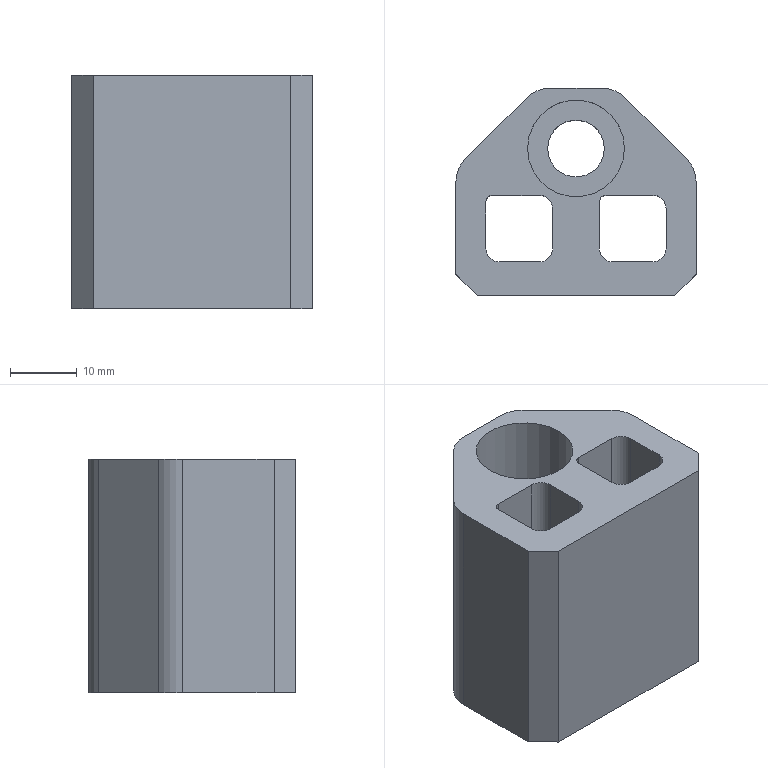Part | NX | features DIE-87 2 | 1 solid | 41 faces | box 36 x 31 x 35 mm | volume 23425 mm3 | plane 23 | cylinder 18 | commonest cylinder face diameters 4 x6 6 x4 10 x4 2 x2 8.5 x1 14.5 x1
STEP:
#1=CARTESIAN_POINT('',(4075.486,-827.123,823.716));
#2=VERTEX_POINT('',#1);
#3=CARTESIAN_POINT('',(4079.736,-827.123,823.716));
#4=DIRECTION('',(0.,0.,1.));
#5=DIRECTION('',(-1.,0.,0.));
#6=AXIS2_PLACEMENT_3D('',#3,#4,#5);
#7=CIRCLE('',#6,4.25);
#8=EDGE_CURVE('',#2,#2,#7,.T.);
#9=ORIENTED_EDGE('',*,*,#8,.T.);
#10=EDGE_LOOP('',(#9));
#11=FACE_BOUND('',#10,.T.);
#12=CARTESIAN_POINT('',(4072.272,-819.587,823.716));
#13=VERTEX_POINT('',#12);
#14=CARTESIAN_POINT('',(4063.201,-828.658,823.716));
#15=VERTEX_POINT('',#14);
#16=CARTESIAN_POINT('',(4078.661,-813.198,823.716));
#17=DIRECTION('',(-0.7071,-0.7071,0.));
#18=VECTOR('',#17,1000.);
#19=LINE('',#16,#18);
#20=EDGE_CURVE('',#13,#15,#19,.T.);
#21=ORIENTED_EDGE('',*,*,#20,.F.);
#22=CARTESIAN_POINT('',(4075.807,-818.123,823.716));
#23=VERTEX_POINT('',#22);
#24=CARTESIAN_POINT('',(4075.807,-823.123,823.716));
#25=DIRECTION('',(0.,0.,1.));
#26=DIRECTION('',(-1.,0.,0.));
#27=AXIS2_PLACEMENT_3D('',#24,#25,#26);
#28=CIRCLE('',#27,5.);
#29=EDGE_CURVE('',#23,#13,#28,.T.);
#30=ORIENTED_EDGE('',*,*,#29,.F.);
#31=CARTESIAN_POINT('',(4083.665,-818.123,823.716));
#32=VERTEX_POINT('',#31);
#33=CARTESIAN_POINT('',(4123.586,-818.123,823.716));
#34=DIRECTION('',(1.,0.,0.));
#35=VECTOR('',#34,1000.);
#36=LINE('',#33,#35);
#37=EDGE_CURVE('',#23,#32,#36,.T.);
#38=ORIENTED_EDGE('',*,*,#37,.T.);
#39=CARTESIAN_POINT('',(4087.201,-819.587,823.716));
#40=VERTEX_POINT('',#39);
#41=CARTESIAN_POINT('',(4083.665,-823.123,823.716));
#42=DIRECTION('',(0.,0.,1.));
#43=DIRECTION('',(-1.,0.,0.));
#44=AXIS2_PLACEMENT_3D('',#41,#42,#43);
#45=CIRCLE('',#44,5.);
#46=EDGE_CURVE('',#40,#32,#45,.T.);
#47=ORIENTED_EDGE('',*,*,#46,.F.);
#48=CARTESIAN_POINT('',(4096.272,-828.658,823.716));
#49=VERTEX_POINT('',#48);
#50=CARTESIAN_POINT('',(4124.661,-857.048,823.716));
#51=DIRECTION('',(-0.7071,0.7071,0.));
#52=VECTOR('',#51,1000.);
#53=LINE('',#50,#52);
#54=EDGE_CURVE('',#49,#40,#53,.T.);
#55=ORIENTED_EDGE('',*,*,#54,.F.);
#56=CARTESIAN_POINT('',(4097.736,-832.194,823.716));
#57=VERTEX_POINT('',#56);
#58=CARTESIAN_POINT('',(4092.736,-832.194,823.716));
#59=DIRECTION('',(0.,0.,1.));
#60=DIRECTION('',(-1.,0.,0.));
#61=AXIS2_PLACEMENT_3D('',#58,#59,#60);
#62=CIRCLE('',#61,5.);
#63=EDGE_CURVE('',#57,#49,#62,.T.);
#64=ORIENTED_EDGE('',*,*,#63,.F.);
#65=CARTESIAN_POINT('',(4097.736,-845.923,823.716));
#66=VERTEX_POINT('',#65);
#67=CARTESIAN_POINT('',(4097.736,-858.123,823.716));
#68=DIRECTION('',(0.,-1.,0.));
#69=VECTOR('',#68,1000.);
#70=LINE('',#67,#69);
#71=EDGE_CURVE('',#57,#66,#70,.T.);
#72=ORIENTED_EDGE('',*,*,#71,.T.);
#73=CARTESIAN_POINT('',(4094.536,-849.123,823.716));
#74=VERTEX_POINT('',#73);
#75=CARTESIAN_POINT('',(4104.561,-839.098,823.716));
#76=DIRECTION('',(-0.7071,-0.7071,0.));
#77=VECTOR('',#76,1000.);
#78=LINE('',#75,#77);
#79=EDGE_CURVE('',#74,#66,#78,.F.);
#80=ORIENTED_EDGE('',*,*,#79,.F.);
#81=CARTESIAN_POINT('',(4064.936,-849.123,823.716));
#82=VERTEX_POINT('',#81);
#83=CARTESIAN_POINT('',(4123.586,-849.123,823.716));
#84=DIRECTION('',(1.,0.,0.));
#85=VECTOR('',#84,1000.);
#86=LINE('',#83,#85);
#87=EDGE_CURVE('',#82,#74,#86,.T.);
#88=ORIENTED_EDGE('',*,*,#87,.F.);
#89=CARTESIAN_POINT('',(4061.736,-845.923,823.716));
#90=VERTEX_POINT('',#89);
#91=CARTESIAN_POINT('',(4098.761,-882.948,823.716));
#92=DIRECTION('',(-0.7071,0.7071,0.));
#93=VECTOR('',#92,1000.);
#94=LINE('',#91,#93);
#95=EDGE_CURVE('',#90,#82,#94,.F.);
#96=ORIENTED_EDGE('',*,*,#95,.F.);
#97=CARTESIAN_POINT('',(4061.736,-832.194,823.716));
#98=VERTEX_POINT('',#97);
#99=CARTESIAN_POINT('',(4061.736,-858.123,823.716));
#100=DIRECTION('',(0.,1.,0.));
#101=VECTOR('',#100,1000.);
#102=LINE('',#99,#101);
#103=EDGE_CURVE('',#90,#98,#102,.T.);
#104=ORIENTED_EDGE('',*,*,#103,.T.);
#105=CARTESIAN_POINT('',(4066.736,-832.194,823.716));
#106=DIRECTION('',(0.,0.,1.));
#107=DIRECTION('',(-1.,0.,0.));
#108=AXIS2_PLACEMENT_3D('',#105,#106,#107);
#109=CIRCLE('',#108,5.);
#110=EDGE_CURVE('',#15,#98,#109,.T.);
#111=ORIENTED_EDGE('',*,*,#110,.F.);
#112=EDGE_LOOP('',(#21,#30,#38,#47,#55,#64,#72,#80,#88,#96,#104,#111));
#113=FACE_BOUND('',#112,.T.);
#114=CARTESIAN_POINT('',(4095.236,-841.123,823.716));
#115=VERTEX_POINT('',#114);
#116=CARTESIAN_POINT('',(4095.236,-837.123,823.716));
#117=VERTEX_POINT('',#116);
#118=CARTESIAN_POINT('',(4095.236,-841.123,823.716));
#119=DIRECTION('',(0.,1.,0.));
#120=VECTOR('',#119,1000.);
#121=LINE('',#118,#120);
#122=EDGE_CURVE('',#115,#117,#121,.T.);
#123=ORIENTED_EDGE('',*,*,#122,.T.);
#124=CARTESIAN_POINT('',(4091.685,-834.174,823.716));
#125=VERTEX_POINT('',#124);
#126=CARTESIAN_POINT('',(4092.236,-837.123,823.716));
#127=DIRECTION('',(0.,0.,1.));
#128=DIRECTION('',(1.,0.,0.));
#129=AXIS2_PLACEMENT_3D('',#126,#127,#128);
#130=CIRCLE('',#129,3.);
#131=EDGE_CURVE('',#117,#125,#130,.T.);
#132=ORIENTED_EDGE('',*,*,#131,.T.);
#133=CARTESIAN_POINT('',(4091.236,-834.123,823.716));
#134=VERTEX_POINT('',#133);
#135=CARTESIAN_POINT('',(4091.236,-836.123,823.716));
#136=DIRECTION('',(0.,0.,-1.));
#137=DIRECTION('',(-1.,0.,0.));
#138=AXIS2_PLACEMENT_3D('',#135,#136,#137);
#139=CIRCLE('',#138,2.);
#140=EDGE_CURVE('',#134,#125,#139,.T.);
#141=ORIENTED_EDGE('',*,*,#140,.F.);
#142=CARTESIAN_POINT('',(4084.236,-834.123,823.716));
#143=VERTEX_POINT('',#142);
#144=CARTESIAN_POINT('',(4088.236,-834.123,823.716));
#145=DIRECTION('',(-1.,0.,0.));
#146=VECTOR('',#145,1000.);
#147=LINE('',#144,#146);
#148=EDGE_CURVE('',#134,#143,#147,.T.);
#149=ORIENTED_EDGE('',*,*,#148,.T.);
#150=CARTESIAN_POINT('',(4083.236,-835.123,823.716));
#151=VERTEX_POINT('',#150);
#152=CARTESIAN_POINT('',(4084.236,-835.123,823.716));
#153=DIRECTION('',(0.,0.,-1.));
#154=DIRECTION('',(-1.,0.,0.));
#155=AXIS2_PLACEMENT_3D('',#152,#153,#154);
#156=CIRCLE('',#155,1.);
#157=EDGE_CURVE('',#151,#143,#156,.T.);
#158=ORIENTED_EDGE('',*,*,#157,.F.);
#159=CARTESIAN_POINT('',(4083.236,-842.123,823.716));
#160=VERTEX_POINT('',#159);
#161=CARTESIAN_POINT('',(4083.236,-839.123,823.716));
#162=DIRECTION('',(0.,-1.,0.));
#163=VECTOR('',#162,1000.);
#164=LINE('',#161,#163);
#165=EDGE_CURVE('',#151,#160,#164,.T.);
#166=ORIENTED_EDGE('',*,*,#165,.T.);
#167=CARTESIAN_POINT('',(4085.236,-844.123,823.716));
#168=VERTEX_POINT('',#167);
#169=CARTESIAN_POINT('',(4085.236,-842.123,823.716));
#170=DIRECTION('',(0.,0.,-1.));
#171=DIRECTION('',(-1.,0.,0.));
#172=AXIS2_PLACEMENT_3D('',#169,#170,#171);
#173=CIRCLE('',#172,2.);
#174=EDGE_CURVE('',#168,#160,#173,.T.);
#175=ORIENTED_EDGE('',*,*,#174,.F.);
#176=CARTESIAN_POINT('',(4091.236,-844.123,823.716));
#177=VERTEX_POINT('',#176);
#178=CARTESIAN_POINT('',(4088.236,-844.123,823.716));
#179=DIRECTION('',(1.,0.,0.));
#180=VECTOR('',#179,1000.);
#181=LINE('',#178,#180);
#182=EDGE_CURVE('',#168,#177,#181,.T.);
#183=ORIENTED_EDGE('',*,*,#182,.T.);
#184=CARTESIAN_POINT('',(4091.685,-844.072,823.716));
#185=VERTEX_POINT('',#184);
#186=CARTESIAN_POINT('',(4091.236,-842.123,823.716));
#187=DIRECTION('',(0.,0.,-1.));
#188=DIRECTION('',(-1.,0.,0.));
#189=AXIS2_PLACEMENT_3D('',#186,#187,#188);
#190=CIRCLE('',#189,2.);
#191=EDGE_CURVE('',#185,#177,#190,.T.);
#192=ORIENTED_EDGE('',*,*,#191,.F.);
#193=CARTESIAN_POINT('',(4092.236,-841.123,823.716));
#194=DIRECTION('',(0.,0.,1.));
#195=DIRECTION('',(1.,0.,0.));
#196=AXIS2_PLACEMENT_3D('',#193,#194,#195);
#197=CIRCLE('',#196,3.);
#198=EDGE_CURVE('',#185,#115,#197,.T.);
#199=ORIENTED_EDGE('',*,*,#198,.T.);
#200=EDGE_LOOP('',(#123,#132,#141,#149,#158,#166,#175,#183,#192,#199));
#201=FACE_BOUND('',#200,.T.);
#202=CARTESIAN_POINT('',(4078.236,-841.123,823.716));
#203=VERTEX_POINT('',#202);
#204=CARTESIAN_POINT('',(4078.236,-837.123,823.716));
#205=VERTEX_POINT('',#204);
#206=CARTESIAN_POINT('',(4078.236,-841.123,823.716));
#207=DIRECTION('',(0.,1.,0.));
#208=VECTOR('',#207,1000.);
#209=LINE('',#206,#208);
#210=EDGE_CURVE('',#203,#205,#209,.T.);
#211=ORIENTED_EDGE('',*,*,#210,.T.);
#212=CARTESIAN_POINT('',(4074.685,-834.174,823.716));
#213=VERTEX_POINT('',#212);
#214=CARTESIAN_POINT('',(4075.236,-837.123,823.716));
#215=DIRECTION('',(0.,0.,1.));
#216=DIRECTION('',(1.,0.,0.));
#217=AXIS2_PLACEMENT_3D('',#214,#215,#216);
#218=CIRCLE('',#217,3.);
#219=EDGE_CURVE('',#205,#213,#218,.T.);
#220=ORIENTED_EDGE('',*,*,#219,.T.);
#221=CARTESIAN_POINT('',(4074.236,-834.123,823.716));
#222=VERTEX_POINT('',#221);
#223=CARTESIAN_POINT('',(4074.236,-836.123,823.716));
#224=DIRECTION('',(0.,0.,-1.));
#225=DIRECTION('',(-1.,0.,0.));
#226=AXIS2_PLACEMENT_3D('',#223,#224,#225);
#227=CIRCLE('',#226,2.);
#228=EDGE_CURVE('',#222,#213,#227,.T.);
#229=ORIENTED_EDGE('',*,*,#228,.F.);
#230=CARTESIAN_POINT('',(4067.236,-834.123,823.716));
#231=VERTEX_POINT('',#230);
#232=CARTESIAN_POINT('',(4071.236,-834.123,823.716));
#233=DIRECTION('',(-1.,0.,0.));
#234=VECTOR('',#233,1000.);
#235=LINE('',#232,#234);
#236=EDGE_CURVE('',#222,#231,#235,.T.);
#237=ORIENTED_EDGE('',*,*,#236,.T.);
#238=CARTESIAN_POINT('',(4066.236,-835.123,823.716));
#239=VERTEX_POINT('',#238);
#240=CARTESIAN_POINT('',(4067.236,-835.123,823.716));
#241=DIRECTION('',(0.,0.,-1.));
#242=DIRECTION('',(-1.,0.,0.));
#243=AXIS2_PLACEMENT_3D('',#240,#241,#242);
#244=CIRCLE('',#243,1.);
#245=EDGE_CURVE('',#239,#231,#244,.T.);
#246=ORIENTED_EDGE('',*,*,#245,.F.);
#247=CARTESIAN_POINT('',(4066.236,-842.123,823.716));
#248=VERTEX_POINT('',#247);
#249=CARTESIAN_POINT('',(4066.236,-839.123,823.716));
#250=DIRECTION('',(0.,-1.,0.));
#251=VECTOR('',#250,1000.);
#252=LINE('',#249,#251);
#253=EDGE_CURVE('',#239,#248,#252,.T.);
#254=ORIENTED_EDGE('',*,*,#253,.T.);
#255=CARTESIAN_POINT('',(4068.236,-844.123,823.716));
#256=VERTEX_POINT('',#255);
#257=CARTESIAN_POINT('',(4068.236,-842.123,823.716));
#258=DIRECTION('',(0.,0.,-1.));
#259=DIRECTION('',(-1.,0.,0.));
#260=AXIS2_PLACEMENT_3D('',#257,#258,#259);
#261=CIRCLE('',#260,2.);
#262=EDGE_CURVE('',#256,#248,#261,.T.);
#263=ORIENTED_EDGE('',*,*,#262,.F.);
#264=CARTESIAN_POINT('',(4074.236,-844.123,823.716));
#265=VERTEX_POINT('',#264);
#266=CARTESIAN_POINT('',(4071.236,-844.123,823.716));
#267=DIRECTION('',(1.,0.,0.));
#268=VECTOR('',#267,1000.);
#269=LINE('',#266,#268);
#270=EDGE_CURVE('',#256,#265,#269,.T.);
#271=ORIENTED_EDGE('',*,*,#270,.T.);
#272=CARTESIAN_POINT('',(4074.685,-844.072,823.716));
#273=VERTEX_POINT('',#272);
#274=CARTESIAN_POINT('',(4074.236,-842.123,823.716));
#275=DIRECTION('',(0.,0.,-1.));
#276=DIRECTION('',(-1.,0.,0.));
#277=AXIS2_PLACEMENT_3D('',#274,#275,#276);
#278=CIRCLE('',#277,2.);
#279=EDGE_CURVE('',#273,#265,#278,.T.);
#280=ORIENTED_EDGE('',*,*,#279,.F.);
#281=CARTESIAN_POINT('',(4075.236,-841.123,823.716));
#282=DIRECTION('',(0.,0.,1.));
#283=DIRECTION('',(1.,0.,0.));
#284=AXIS2_PLACEMENT_3D('',#281,#282,#283);
#285=CIRCLE('',#284,3.);
#286=EDGE_CURVE('',#273,#203,#285,.T.);
#287=ORIENTED_EDGE('',*,*,#286,.T.);
#288=EDGE_LOOP('',(#211,#220,#229,#237,#246,#254,#263,#271,#280,#287));
#289=FACE_BOUND('',#288,.T.);
#290=CARTESIAN_POINT('',(4123.586,-858.123,823.716));
#291=DIRECTION('',(0.,0.,-1.));
#292=DIRECTION('',(-1.,0.,0.));
#293=AXIS2_PLACEMENT_3D('',#290,#291,#292);
#294=PLANE('',#293);
#295=ADVANCED_FACE('',(#11,#113,#201,#289),#294,.T.);
#296=CARTESIAN_POINT('',(4074.685,-834.174,828.716));
#297=VERTEX_POINT('',#296);
#298=CARTESIAN_POINT('',(4074.685,-834.174,826.216));
#299=DIRECTION('',(0.,0.,-1.));
#300=VECTOR('',#299,1000.);
#301=LINE('',#298,#300);
#302=EDGE_CURVE('',#297,#213,#301,.T.);
#303=ORIENTED_EDGE('',*,*,#302,.F.);
#304=CARTESIAN_POINT('',(4076.236,-836.123,828.716));
#305=VERTEX_POINT('',#304);
#306=CARTESIAN_POINT('',(4074.236,-836.123,828.716));
#307=DIRECTION('',(0.,0.,1.));
#308=DIRECTION('',(1.,0.,0.));
#309=AXIS2_PLACEMENT_3D('',#306,#307,#308);
#310=CIRCLE('',#309,2.);
#311=EDGE_CURVE('',#297,#305,#310,.F.);
#312=ORIENTED_EDGE('',*,*,#311,.T.);
#313=CARTESIAN_POINT('',(4076.236,-836.123,858.716));
#314=VERTEX_POINT('',#313);
#315=CARTESIAN_POINT('',(4076.236,-836.123,823.716));
#316=DIRECTION('',(0.,0.,1.));
#317=VECTOR('',#316,1000.);
#318=LINE('',#315,#317);
#319=EDGE_CURVE('',#314,#305,#318,.F.);
#320=ORIENTED_EDGE('',*,*,#319,.F.);
#321=CARTESIAN_POINT('',(4074.236,-834.123,858.716));
#322=VERTEX_POINT('',#321);
#323=CARTESIAN_POINT('',(4074.236,-836.123,858.716));
#324=DIRECTION('',(0.,0.,1.));
#325=DIRECTION('',(1.,0.,0.));
#326=AXIS2_PLACEMENT_3D('',#323,#324,#325);
#327=CIRCLE('',#326,2.);
#328=EDGE_CURVE('',#314,#322,#327,.T.);
#329=ORIENTED_EDGE('',*,*,#328,.T.);
#330=CARTESIAN_POINT('',(4074.236,-834.123,823.716));
#331=DIRECTION('',(0.,0.,1.));
#332=VECTOR('',#331,1000.);
#333=LINE('',#330,#332);
#334=EDGE_CURVE('',#222,#322,#333,.T.);
#335=ORIENTED_EDGE('',*,*,#334,.F.);
#336=ORIENTED_EDGE('',*,*,#228,.T.);
#337=EDGE_LOOP('',(#303,#312,#320,#329,#335,#336));
#338=FACE_BOUND('',#337,.T.);
#339=CARTESIAN_POINT('',(4074.236,-836.123,823.716));
#340=DIRECTION('',(0.,0.,1.));
#341=DIRECTION('',(1.,0.,0.));
#342=AXIS2_PLACEMENT_3D('',#339,#340,#341);
#343=CYLINDRICAL_SURFACE('',#342,2.);
#344=ADVANCED_FACE('',(#338),#343,.F.);
#345=CARTESIAN_POINT('',(4074.685,-844.072,828.716));
#346=VERTEX_POINT('',#345);
#347=CARTESIAN_POINT('',(4074.685,-844.072,826.216));
#348=DIRECTION('',(0.,0.,-1.));
#349=VECTOR('',#348,1000.);
#350=LINE('',#347,#349);
#351=EDGE_CURVE('',#273,#346,#350,.F.);
#352=ORIENTED_EDGE('',*,*,#351,.F.);
#353=ORIENTED_EDGE('',*,*,#279,.T.);
#354=CARTESIAN_POINT('',(4074.236,-844.123,858.716));
#355=VERTEX_POINT('',#354);
#356=CARTESIAN_POINT('',(4074.236,-844.123,823.716));
#357=DIRECTION('',(0.,0.,1.));
#358=VECTOR('',#357,1000.);
#359=LINE('',#356,#358);
#360=EDGE_CURVE('',#355,#265,#359,.F.);
#361=ORIENTED_EDGE('',*,*,#360,.F.);
#362=CARTESIAN_POINT('',(4076.236,-842.123,858.716));
#363=VERTEX_POINT('',#362);
#364=CARTESIAN_POINT('',(4074.236,-842.123,858.716));
#365=DIRECTION('',(0.,0.,1.));
#366=DIRECTION('',(1.,0.,0.));
#367=AXIS2_PLACEMENT_3D('',#364,#365,#366);
#368=CIRCLE('',#367,2.);
#369=EDGE_CURVE('',#355,#363,#368,.T.);
#370=ORIENTED_EDGE('',*,*,#369,.T.);
#371=CARTESIAN_POINT('',(4076.236,-842.123,828.716));
#372=VERTEX_POINT('',#371);
#373=CARTESIAN_POINT('',(4076.236,-842.123,823.716));
#374=DIRECTION('',(0.,0.,1.));
#375=VECTOR('',#374,1000.);
#376=LINE('',#373,#375);
#377=EDGE_CURVE('',#372,#363,#376,.T.);
#378=ORIENTED_EDGE('',*,*,#377,.F.);
#379=CARTESIAN_POINT('',(4074.236,-842.123,828.716));
#380=DIRECTION('',(0.,0.,1.));
#381=DIRECTION('',(1.,0.,0.));
#382=AXIS2_PLACEMENT_3D('',#379,#380,#381);
#383=CIRCLE('',#382,2.);
#384=EDGE_CURVE('',#372,#346,#383,.F.);
#385=ORIENTED_EDGE('',*,*,#384,.T.);
#386=EDGE_LOOP('',(#352,#353,#361,#370,#378,#385));
#387=FACE_BOUND('',#386,.T.);
#388=CARTESIAN_POINT('',(4074.236,-842.123,823.716));
#389=DIRECTION('',(0.,0.,1.));
#390=DIRECTION('',(1.,0.,0.));
#391=AXIS2_PLACEMENT_3D('',#388,#389,#390);
#392=CYLINDRICAL_SURFACE('',#391,2.);
#393=ADVANCED_FACE('',(#387),#392,.F.);
#394=CARTESIAN_POINT('',(4091.685,-834.174,828.716));
#395=VERTEX_POINT('',#394);
#396=CARTESIAN_POINT('',(4091.685,-834.174,826.216));
#397=DIRECTION('',(0.,0.,-1.));
#398=VECTOR('',#397,1000.);
#399=LINE('',#396,#398);
#400=EDGE_CURVE('',#395,#125,#399,.T.);
#401=ORIENTED_EDGE('',*,*,#400,.F.);
#402=CARTESIAN_POINT('',(4093.236,-836.123,828.716));
#403=VERTEX_POINT('',#402);
#404=CARTESIAN_POINT('',(4091.236,-836.123,828.716));
#405=DIRECTION('',(0.,0.,1.));
#406=DIRECTION('',(1.,0.,0.));
#407=AXIS2_PLACEMENT_3D('',#404,#405,#406);
#408=CIRCLE('',#407,2.);
#409=EDGE_CURVE('',#395,#403,#408,.F.);
#410=ORIENTED_EDGE('',*,*,#409,.T.);
#411=CARTESIAN_POINT('',(4093.236,-836.123,858.716));
#412=VERTEX_POINT('',#411);
#413=CARTESIAN_POINT('',(4093.236,-836.123,823.716));
#414=DIRECTION('',(0.,0.,1.));
#415=VECTOR('',#414,1000.);
#416=LINE('',#413,#415);
#417=EDGE_CURVE('',#412,#403,#416,.F.);
#418=ORIENTED_EDGE('',*,*,#417,.F.);
#419=CARTESIAN_POINT('',(4091.236,-834.123,858.716));
#420=VERTEX_POINT('',#419);
#421=CARTESIAN_POINT('',(4091.236,-836.123,858.716));
#422=DIRECTION('',(0.,0.,1.));
#423=DIRECTION('',(1.,0.,0.));
#424=AXIS2_PLACEMENT_3D('',#421,#422,#423);
#425=CIRCLE('',#424,2.);
#426=EDGE_CURVE('',#412,#420,#425,.T.);
#427=ORIENTED_EDGE('',*,*,#426,.T.);
#428=CARTESIAN_POINT('',(4091.236,-834.123,823.716));
#429=DIRECTION('',(0.,0.,1.));
#430=VECTOR('',#429,1000.);
#431=LINE('',#428,#430);
#432=EDGE_CURVE('',#134,#420,#431,.T.);
#433=ORIENTED_EDGE('',*,*,#432,.F.);
#434=ORIENTED_EDGE('',*,*,#140,.T.);
#435=EDGE_LOOP('',(#401,#410,#418,#427,#433,#434));
#436=FACE_BOUND('',#435,.T.);
#437=CARTESIAN_POINT('',(4091.236,-836.123,823.716));
#438=DIRECTION('',(0.,0.,1.));
#439=DIRECTION('',(1.,0.,0.));
#440=AXIS2_PLACEMENT_3D('',#437,#438,#439);
#441=CYLINDRICAL_SURFACE('',#440,2.);
#442=ADVANCED_FACE('',(#436),#441,.F.);
#443=CARTESIAN_POINT('',(4091.685,-844.072,828.716));
#444=VERTEX_POINT('',#443);
#445=CARTESIAN_POINT('',(4091.685,-844.072,826.216));
#446=DIRECTION('',(0.,0.,-1.));
#447=VECTOR('',#446,1000.);
#448=LINE('',#445,#447);
#449=EDGE_CURVE('',#185,#444,#448,.F.);
#450=ORIENTED_EDGE('',*,*,#449,.F.);
#451=ORIENTED_EDGE('',*,*,#191,.T.);
#452=CARTESIAN_POINT('',(4091.236,-844.123,858.716));
#453=VERTEX_POINT('',#452);
#454=CARTESIAN_POINT('',(4091.236,-844.123,823.716));
#455=DIRECTION('',(0.,0.,1.));
#456=VECTOR('',#455,1000.);
#457=LINE('',#454,#456);
#458=EDGE_CURVE('',#453,#177,#457,.F.);
#459=ORIENTED_EDGE('',*,*,#458,.F.);
#460=CARTESIAN_POINT('',(4093.236,-842.123,858.716));
#461=VERTEX_POINT('',#460);
#462=CARTESIAN_POINT('',(4091.236,-842.123,858.716));
#463=DIRECTION('',(0.,0.,1.));
#464=DIRECTION('',(1.,0.,0.));
#465=AXIS2_PLACEMENT_3D('',#462,#463,#464);
#466=CIRCLE('',#465,2.);
#467=EDGE_CURVE('',#453,#461,#466,.T.);
#468=ORIENTED_EDGE('',*,*,#467,.T.);
#469=CARTESIAN_POINT('',(4093.236,-842.123,828.716));
#470=VERTEX_POINT('',#469);
#471=CARTESIAN_POINT('',(4093.236,-842.123,823.716));
#472=DIRECTION('',(0.,0.,1.));
#473=VECTOR('',#472,1000.);
#474=LINE('',#471,#473);
#475=EDGE_CURVE('',#470,#461,#474,.T.);
#476=ORIENTED_EDGE('',*,*,#475,.F.);
#477=CARTESIAN_POINT('',(4091.236,-842.123,828.716));
#478=DIRECTION('',(0.,0.,1.));
#479=DIRECTION('',(1.,0.,0.));
#480=AXIS2_PLACEMENT_3D('',#477,#478,#479);
#481=CIRCLE('',#480,2.);
#482=EDGE_CURVE('',#470,#444,#481,.F.);
#483=ORIENTED_EDGE('',*,*,#482,.T.);
#484=EDGE_LOOP('',(#450,#451,#459,#468,#476,#483));
#485=FACE_BOUND('',#484,.T.);
#486=CARTESIAN_POINT('',(4091.236,-842.123,823.716));
#487=DIRECTION('',(0.,0.,1.));
#488=DIRECTION('',(1.,0.,0.));
#489=AXIS2_PLACEMENT_3D('',#486,#487,#488);
#490=CYLINDRICAL_SURFACE('',#489,2.);
#491=ADVANCED_FACE('',(#485),#490,.F.);
#492=CARTESIAN_POINT('',(4064.936,-849.123,858.716));
#493=VERTEX_POINT('',#492);
#494=CARTESIAN_POINT('',(4094.536,-849.123,858.716));
#495=VERTEX_POINT('',#494);
#496=CARTESIAN_POINT('',(4079.736,-849.123,858.716));
#497=DIRECTION('',(-1.,0.,0.));
#498=VECTOR('',#497,1000.);
#499=LINE('',#496,#498);
#500=EDGE_CURVE('',#493,#495,#499,.F.);
#501=ORIENTED_EDGE('',*,*,#500,.F.);
#502=CARTESIAN_POINT('',(4064.936,-849.123,858.716));
#503=DIRECTION('',(0.,0.,1.));
#504=VECTOR('',#503,1000.);
#505=LINE('',#502,#504);
#506=EDGE_CURVE('',#82,#493,#505,.T.);
#507=ORIENTED_EDGE('',*,*,#506,.F.);
#508=ORIENTED_EDGE('',*,*,#87,.T.);
#509=CARTESIAN_POINT('',(4094.536,-849.123,858.716));
#510=DIRECTION('',(0.,0.,-1.));
#511=VECTOR('',#510,1000.);
#512=LINE('',#509,#511);
#513=EDGE_CURVE('',#495,#74,#512,.T.);
#514=ORIENTED_EDGE('',*,*,#513,.F.);
#515=EDGE_LOOP('',(#501,#507,#508,#514));
#516=FACE_BOUND('',#515,.T.);
#517=CARTESIAN_POINT('',(4088.236,-849.123,858.716));
#518=DIRECTION('',(0.,-1.,0.));
#519=DIRECTION('',(0.,0.,1.));
#520=AXIS2_PLACEMENT_3D('',#517,#518,#519);
#521=PLANE('',#520);
#522=ADVANCED_FACE('',(#516),#521,.T.);
#523=CARTESIAN_POINT('',(4083.236,-842.123,858.716));
#524=VERTEX_POINT('',#523);
#525=CARTESIAN_POINT('',(4085.236,-844.123,858.716));
#526=VERTEX_POINT('',#525);
#527=CARTESIAN_POINT('',(4085.236,-842.123,858.716));
#528=DIRECTION('',(0.,0.,1.));
#529=DIRECTION('',(1.,0.,0.));
#530=AXIS2_PLACEMENT_3D('',#527,#528,#529);
#531=CIRCLE('',#530,2.);
#532=EDGE_CURVE('',#524,#526,#531,.T.);
#533=ORIENTED_EDGE('',*,*,#532,.F.);
#534=CARTESIAN_POINT('',(4083.236,-835.123,858.716));
#535=VERTEX_POINT('',#534);
#536=CARTESIAN_POINT('',(4083.236,-839.123,858.716));
#537=DIRECTION('',(0.,1.,0.));
#538=VECTOR('',#537,1000.);
#539=LINE('',#536,#538);
#540=EDGE_CURVE('',#524,#535,#539,.T.);
#541=ORIENTED_EDGE('',*,*,#540,.T.);
#542=CARTESIAN_POINT('',(4084.236,-834.123,858.716));
#543=VERTEX_POINT('',#542);
#544=CARTESIAN_POINT('',(4084.236,-835.123,858.716));
#545=DIRECTION('',(0.,0.,1.));
#546=DIRECTION('',(1.,0.,0.));
#547=AXIS2_PLACEMENT_3D('',#544,#545,#546);
#548=CIRCLE('',#547,1.);
#549=EDGE_CURVE('',#543,#535,#548,.T.);
#550=ORIENTED_EDGE('',*,*,#549,.F.);
#551=CARTESIAN_POINT('',(4088.236,-834.123,858.716));
#552=DIRECTION('',(1.,0.,0.));
#553=VECTOR('',#552,1000.);
#554=LINE('',#551,#553);
#555=EDGE_CURVE('',#543,#420,#554,.T.);
#556=ORIENTED_EDGE('',*,*,#555,.T.);
#557=ORIENTED_EDGE('',*,*,#426,.F.);
#558=CARTESIAN_POINT('',(4093.236,-839.123,858.716));
#559=DIRECTION('',(0.,-1.,0.));
#560=VECTOR('',#559,1000.);
#561=LINE('',#558,#560);
#562=EDGE_CURVE('',#412,#461,#561,.T.);
#563=ORIENTED_EDGE('',*,*,#562,.T.);
#564=ORIENTED_EDGE('',*,*,#467,.F.);
#565=CARTESIAN_POINT('',(4088.236,-844.123,858.716));
#566=DIRECTION('',(-1.,0.,0.));
#567=VECTOR('',#566,1000.);
#568=LINE('',#565,#567);
#569=EDGE_CURVE('',#453,#526,#568,.T.);
#570=ORIENTED_EDGE('',*,*,#569,.T.);
#571=EDGE_LOOP('',(#533,#541,#550,#556,#557,#563,#564,#570));
#572=FACE_BOUND('',#571,.T.);
#573=CARTESIAN_POINT('',(4066.236,-842.123,858.716));
#574=VERTEX_POINT('',#573);
#575=CARTESIAN_POINT('',(4068.236,-844.123,858.716));
#576=VERTEX_POINT('',#575);
#577=CARTESIAN_POINT('',(4068.236,-842.123,858.716));
#578=DIRECTION('',(0.,0.,1.));
#579=DIRECTION('',(1.,0.,0.));
#580=AXIS2_PLACEMENT_3D('',#577,#578,#579);
#581=CIRCLE('',#580,2.);
#582=EDGE_CURVE('',#574,#576,#581,.T.);
#583=ORIENTED_EDGE('',*,*,#582,.F.);
#584=CARTESIAN_POINT('',(4066.236,-835.123,858.716));
#585=VERTEX_POINT('',#584);
#586=CARTESIAN_POINT('',(4066.236,-839.123,858.716));
#587=DIRECTION('',(0.,1.,0.));
#588=VECTOR('',#587,1000.);
#589=LINE('',#586,#588);
#590=EDGE_CURVE('',#574,#585,#589,.T.);
#591=ORIENTED_EDGE('',*,*,#590,.T.);
#592=CARTESIAN_POINT('',(4067.236,-834.123,858.716));
#593=VERTEX_POINT('',#592);
#594=CARTESIAN_POINT('',(4067.236,-835.123,858.716));
#595=DIRECTION('',(0.,0.,1.));
#596=DIRECTION('',(1.,0.,0.));
#597=AXIS2_PLACEMENT_3D('',#594,#595,#596);
#598=CIRCLE('',#597,1.);
#599=EDGE_CURVE('',#593,#585,#598,.T.);
#600=ORIENTED_EDGE('',*,*,#599,.F.);
#601=CARTESIAN_POINT('',(4071.236,-834.123,858.716));
#602=DIRECTION('',(1.,0.,0.));
#603=VECTOR('',#602,1000.);
#604=LINE('',#601,#603);
#605=EDGE_CURVE('',#593,#322,#604,.T.);
#606=ORIENTED_EDGE('',*,*,#605,.T.);
#607=ORIENTED_EDGE('',*,*,#328,.F.);
#608=CARTESIAN_POINT('',(4076.236,-839.123,858.716));
#609=DIRECTION('',(0.,-1.,0.));
#610=VECTOR('',#609,1000.);
#611=LINE('',#608,#610);
#612=EDGE_CURVE('',#314,#363,#611,.T.);
#613=ORIENTED_EDGE('',*,*,#612,.T.);
#614=ORIENTED_EDGE('',*,*,#369,.F.);
#615=CARTESIAN_POINT('',(4071.236,-844.123,858.716));
#616=DIRECTION('',(-1.,0.,0.));
#617=VECTOR('',#616,1000.);
#618=LINE('',#615,#617);
#619=EDGE_CURVE('',#355,#576,#618,.T.);
#620=ORIENTED_EDGE('',*,*,#619,.T.);
#621=EDGE_LOOP('',(#583,#591,#600,#606,#607,#613,#614,#620));
#622=FACE_BOUND('',#621,.T.);
#623=CARTESIAN_POINT('',(4086.986,-827.123,858.716));
#624=VERTEX_POINT('',#623);
#625=CARTESIAN_POINT('',(4079.736,-827.123,858.716));
#626=DIRECTION('',(0.,0.,-1.));
#627=DIRECTION('',(1.,0.,0.));
#628=AXIS2_PLACEMENT_3D('',#625,#626,#627);
#629=CIRCLE('',#628,7.25);
#630=EDGE_CURVE('',#624,#624,#629,.T.);
#631=ORIENTED_EDGE('',*,*,#630,.T.);
#632=EDGE_LOOP('',(#631));
#633=FACE_BOUND('',#632,.T.);
#634=CARTESIAN_POINT('',(4061.736,-832.194,858.716));
#635=VERTEX_POINT('',#634);
#636=CARTESIAN_POINT('',(4061.736,-845.923,858.716));
#637=VERTEX_POINT('',#636);
#638=CARTESIAN_POINT('',(4061.736,-858.123,858.716));
#639=DIRECTION('',(0.,-1.,0.));
#640=VECTOR('',#639,1000.);
#641=LINE('',#638,#640);
#642=EDGE_CURVE('',#635,#637,#641,.T.);
#643=ORIENTED_EDGE('',*,*,#642,.T.);
#644=CARTESIAN_POINT('',(4076.836,-861.023,858.716));
#645=DIRECTION('',(0.7071,-0.7071,0.));
#646=VECTOR('',#645,1000.);
#647=LINE('',#644,#646);
#648=EDGE_CURVE('',#493,#637,#647,.F.);
#649=ORIENTED_EDGE('',*,*,#648,.F.);
#650=ORIENTED_EDGE('',*,*,#500,.T.);
#651=CARTESIAN_POINT('',(4097.736,-845.923,858.716));
#652=VERTEX_POINT('',#651);
#653=CARTESIAN_POINT('',(4082.636,-861.023,858.716));
#654=DIRECTION('',(0.7071,0.7071,0.));
#655=VECTOR('',#654,1000.);
#656=LINE('',#653,#655);
#657=EDGE_CURVE('',#652,#495,#656,.F.);
#658=ORIENTED_EDGE('',*,*,#657,.F.);
#659=CARTESIAN_POINT('',(4097.736,-832.194,858.716));
#660=VERTEX_POINT('',#659);
#661=CARTESIAN_POINT('',(4097.736,-858.123,858.716));
#662=DIRECTION('',(0.,1.,0.));
#663=VECTOR('',#662,1000.);
#664=LINE('',#661,#663);
#665=EDGE_CURVE('',#652,#660,#664,.T.);
#666=ORIENTED_EDGE('',*,*,#665,.T.);
#667=CARTESIAN_POINT('',(4096.272,-828.658,858.716));
#668=VERTEX_POINT('',#667);
#669=CARTESIAN_POINT('',(4092.736,-832.194,858.716));
#670=DIRECTION('',(0.,0.,-1.));
#671=DIRECTION('',(1.,0.,0.));
#672=AXIS2_PLACEMENT_3D('',#669,#670,#671);
#673=CIRCLE('',#672,5.);
#674=EDGE_CURVE('',#668,#660,#673,.T.);
#675=ORIENTED_EDGE('',*,*,#674,.F.);
#676=CARTESIAN_POINT('',(4087.201,-819.587,858.716));
#677=VERTEX_POINT('',#676);
#678=CARTESIAN_POINT('',(4102.736,-835.123,858.716));
#679=DIRECTION('',(0.7071,-0.7071,0.));
#680=VECTOR('',#679,1000.);
#681=LINE('',#678,#680);
#682=EDGE_CURVE('',#677,#668,#681,.T.);
#683=ORIENTED_EDGE('',*,*,#682,.F.);
#684=CARTESIAN_POINT('',(4083.665,-818.123,858.716));
#685=VERTEX_POINT('',#684);
#686=CARTESIAN_POINT('',(4083.665,-823.123,858.716));
#687=DIRECTION('',(0.,0.,-1.));
#688=DIRECTION('',(1.,0.,0.));
#689=AXIS2_PLACEMENT_3D('',#686,#687,#688);
#690=CIRCLE('',#689,5.);
#691=EDGE_CURVE('',#685,#677,#690,.T.);
#692=ORIENTED_EDGE('',*,*,#691,.F.);
#693=CARTESIAN_POINT('',(4075.807,-818.123,858.716));
#694=VERTEX_POINT('',#693);
#695=CARTESIAN_POINT('',(4088.236,-818.123,858.716));
#696=DIRECTION('',(1.,0.,0.));
#697=VECTOR('',#696,1000.);
#698=LINE('',#695,#697);
#699=EDGE_CURVE('',#694,#685,#698,.T.);
#700=ORIENTED_EDGE('',*,*,#699,.F.);
#701=CARTESIAN_POINT('',(4072.272,-819.587,858.716));
#702=VERTEX_POINT('',#701);
#703=CARTESIAN_POINT('',(4075.807,-823.123,858.716));
#704=DIRECTION('',(0.,0.,-1.));
#705=DIRECTION('',(1.,0.,0.));
#706=AXIS2_PLACEMENT_3D('',#703,#704,#705);
#707=CIRCLE('',#706,5.);
#708=EDGE_CURVE('',#702,#694,#707,.T.);
#709=ORIENTED_EDGE('',*,*,#708,.F.);
#710=CARTESIAN_POINT('',(4063.201,-828.658,858.716));
#711=VERTEX_POINT('',#710);
#712=CARTESIAN_POINT('',(4056.736,-835.123,858.716));
#713=DIRECTION('',(0.7071,0.7071,0.));
#714=VECTOR('',#713,1000.);
#715=LINE('',#712,#714);
#716=EDGE_CURVE('',#711,#702,#715,.T.);
#717=ORIENTED_EDGE('',*,*,#716,.F.);
#718=CARTESIAN_POINT('',(4066.736,-832.194,858.716));
#719=DIRECTION('',(0.,0.,-1.));
#720=DIRECTION('',(1.,0.,0.));
#721=AXIS2_PLACEMENT_3D('',#718,#719,#720);
#722=CIRCLE('',#721,5.);
#723=EDGE_CURVE('',#635,#711,#722,.T.);
#724=ORIENTED_EDGE('',*,*,#723,.F.);
#725=EDGE_LOOP('',(#643,#649,#650,#658,#666,#675,#683,#692,#700,#709,#717,#724));
#726=FACE_BOUND('',#725,.T.);
#727=CARTESIAN_POINT('',(4079.736,-858.123,858.716));
#728=DIRECTION('',(0.,0.,1.));
#729=DIRECTION('',(1.,0.,0.));
#730=AXIS2_PLACEMENT_3D('',#727,#728,#729);
#731=PLANE('',#730);
#732=ADVANCED_FACE('',(#572,#622,#633,#726),#731,.T.);
#733=ORIENTED_EDGE('',*,*,#665,.F.);
#734=CARTESIAN_POINT('',(4097.736,-845.923,823.716));
#735=DIRECTION('',(0.,0.,1.));
#736=VECTOR('',#735,1000.);
#737=LINE('',#734,#736);
#738=EDGE_CURVE('',#66,#652,#737,.T.);
#739=ORIENTED_EDGE('',*,*,#738,.F.);
#740=ORIENTED_EDGE('',*,*,#71,.F.);
#741=CARTESIAN_POINT('',(4097.736,-832.194,823.716));
#742=DIRECTION('',(0.,0.,-1.));
#743=VECTOR('',#742,1000.);
#744=LINE('',#741,#743);
#745=EDGE_CURVE('',#660,#57,#744,.T.);
#746=ORIENTED_EDGE('',*,*,#745,.F.);
#747=EDGE_LOOP('',(#733,#739,#740,#746));
#748=FACE_BOUND('',#747,.T.);
#749=CARTESIAN_POINT('',(4097.736,-858.123,823.716));
#750=DIRECTION('',(1.,0.,0.));
#751=DIRECTION('',(0.,0.,-1.));
#752=AXIS2_PLACEMENT_3D('',#749,#750,#751);
#753=PLANE('',#752);
#754=ADVANCED_FACE('',(#748),#753,.T.);
#755=ORIENTED_EDGE('',*,*,#103,.F.);
#756=CARTESIAN_POINT('',(4061.736,-845.923,823.716));
#757=DIRECTION('',(0.,0.,-1.));
#758=VECTOR('',#757,1000.);
#759=LINE('',#756,#758);
#760=EDGE_CURVE('',#637,#90,#759,.T.);
#761=ORIENTED_EDGE('',*,*,#760,.F.);
#762=ORIENTED_EDGE('',*,*,#642,.F.);
#763=CARTESIAN_POINT('',(4061.736,-832.194,823.716));
#764=DIRECTION('',(0.,0.,1.));
#765=VECTOR('',#764,1000.);
#766=LINE('',#763,#765);
#767=EDGE_CURVE('',#98,#635,#766,.T.);
#768=ORIENTED_EDGE('',*,*,#767,.F.);
#769=EDGE_LOOP('',(#755,#761,#762,#768));
#770=FACE_BOUND('',#769,.T.);
#771=CARTESIAN_POINT('',(4061.736,-858.123,823.716));
#772=DIRECTION('',(-1.,0.,0.));
#773=DIRECTION('',(0.,0.,1.));
#774=AXIS2_PLACEMENT_3D('',#771,#772,#773);
#775=PLANE('',#774);
#776=ADVANCED_FACE('',(#770),#775,.T.);
#777=ORIENTED_EDGE('',*,*,#37,.F.);
#778=CARTESIAN_POINT('',(4075.807,-818.123,823.716));
#779=DIRECTION('',(0.,0.,-1.));
#780=VECTOR('',#779,1000.);
#781=LINE('',#778,#780);
#782=EDGE_CURVE('',#694,#23,#781,.T.);
#783=ORIENTED_EDGE('',*,*,#782,.F.);
#784=ORIENTED_EDGE('',*,*,#699,.T.);
#785=CARTESIAN_POINT('',(4083.665,-818.123,858.716));
#786=DIRECTION('',(0.,0.,1.));
#787=VECTOR('',#786,1000.);
#788=LINE('',#785,#787);
#789=EDGE_CURVE('',#32,#685,#788,.T.);
#790=ORIENTED_EDGE('',*,*,#789,.F.);
#791=EDGE_LOOP('',(#777,#783,#784,#790));
#792=FACE_BOUND('',#791,.T.);
#793=CARTESIAN_POINT('',(4088.236,-818.123,858.716));
#794=DIRECTION('',(0.,-1.,0.));
#795=DIRECTION('',(0.,0.,1.));
#796=AXIS2_PLACEMENT_3D('',#793,#794,#795);
#797=PLANE('',#796);
#798=ADVANCED_FACE('',(#792),#797,.F.);
#799=ORIENTED_EDGE('',*,*,#657,.T.);
#800=ORIENTED_EDGE('',*,*,#513,.T.);
#801=ORIENTED_EDGE('',*,*,#79,.T.);
#802=ORIENTED_EDGE('',*,*,#738,.T.);
#803=EDGE_LOOP('',(#799,#800,#801,#802));
#804=FACE_BOUND('',#803,.T.);
#805=CARTESIAN_POINT('',(4094.536,-849.123,858.716));
#806=DIRECTION('',(-0.7071,0.7071,0.));
#807=DIRECTION('',(0.,0.,-1.));
#808=AXIS2_PLACEMENT_3D('',#805,#806,#807);
#809=PLANE('',#808);
#810=ADVANCED_FACE('',(#804),#809,.F.);
#811=ORIENTED_EDGE('',*,*,#95,.T.);
#812=ORIENTED_EDGE('',*,*,#506,.T.);
#813=ORIENTED_EDGE('',*,*,#648,.T.);
#814=ORIENTED_EDGE('',*,*,#760,.T.);
#815=EDGE_LOOP('',(#811,#812,#813,#814));
#816=FACE_BOUND('',#815,.T.);
#817=CARTESIAN_POINT('',(4064.936,-849.123,858.716));
#818=DIRECTION('',(0.7071,0.7071,0.));
#819=DIRECTION('',(0.,0.,1.));
#820=AXIS2_PLACEMENT_3D('',#817,#818,#819);
#821=PLANE('',#820);
#822=ADVANCED_FACE('',(#816),#821,.F.);
#823=ORIENTED_EDGE('',*,*,#54,.T.);
#824=CARTESIAN_POINT('',(4087.201,-819.587,823.716));
#825=DIRECTION('',(0.,0.,1.));
#826=VECTOR('',#825,1000.);
#827=LINE('',#824,#826);
#828=EDGE_CURVE('',#677,#40,#827,.F.);
#829=ORIENTED_EDGE('',*,*,#828,.F.);
#830=ORIENTED_EDGE('',*,*,#682,.T.);
#831=CARTESIAN_POINT('',(4096.272,-828.658,823.716));
#832=DIRECTION('',(0.,0.,-1.));
#833=VECTOR('',#832,1000.);
#834=LINE('',#831,#833);
#835=EDGE_CURVE('',#49,#668,#834,.F.);
#836=ORIENTED_EDGE('',*,*,#835,.F.);
#837=EDGE_LOOP('',(#823,#829,#830,#836));
#838=FACE_BOUND('',#837,.T.);
#839=CARTESIAN_POINT('',(4097.736,-830.123,823.716));
#840=DIRECTION('',(0.7071,0.7071,0.));
#841=DIRECTION('',(0.,0.,1.));
#842=AXIS2_PLACEMENT_3D('',#839,#840,#841);
#843=PLANE('',#842);
#844=ADVANCED_FACE('',(#838),#843,.T.);
#845=ORIENTED_EDGE('',*,*,#716,.T.);
#846=CARTESIAN_POINT('',(4072.272,-819.587,858.716));
#847=DIRECTION('',(0.,0.,-1.));
#848=VECTOR('',#847,1000.);
#849=LINE('',#846,#848);
#850=EDGE_CURVE('',#13,#702,#849,.F.);
#851=ORIENTED_EDGE('',*,*,#850,.F.);
#852=ORIENTED_EDGE('',*,*,#20,.T.);
#853=CARTESIAN_POINT('',(4063.201,-828.658,858.716));
#854=DIRECTION('',(0.,0.,1.));
#855=VECTOR('',#854,1000.);
#856=LINE('',#853,#855);
#857=EDGE_CURVE('',#711,#15,#856,.F.);
#858=ORIENTED_EDGE('',*,*,#857,.F.);
#859=EDGE_LOOP('',(#845,#851,#852,#858));
#860=FACE_BOUND('',#859,.T.);
#861=CARTESIAN_POINT('',(4073.736,-818.123,858.716));
#862=DIRECTION('',(-0.7071,0.7071,0.));
#863=DIRECTION('',(0.,0.,1.));
#864=AXIS2_PLACEMENT_3D('',#861,#862,#863);
#865=PLANE('',#864);
#866=ADVANCED_FACE('',(#860),#865,.T.);
#867=ORIENTED_EDGE('',*,*,#110,.T.);
#868=ORIENTED_EDGE('',*,*,#767,.T.);
#869=ORIENTED_EDGE('',*,*,#723,.T.);
#870=ORIENTED_EDGE('',*,*,#857,.T.);
#871=EDGE_LOOP('',(#867,#868,#869,#870));
#872=FACE_BOUND('',#871,.T.);
#873=CARTESIAN_POINT('',(4066.736,-832.194,823.716));
#874=DIRECTION('',(0.,0.,1.));
#875=DIRECTION('',(1.,0.,0.));
#876=AXIS2_PLACEMENT_3D('',#873,#874,#875);
#877=CYLINDRICAL_SURFACE('',#876,5.);
#878=ADVANCED_FACE('',(#872),#877,.T.);
#879=ORIENTED_EDGE('',*,*,#674,.T.);
#880=ORIENTED_EDGE('',*,*,#745,.T.);
#881=ORIENTED_EDGE('',*,*,#63,.T.);
#882=ORIENTED_EDGE('',*,*,#835,.T.);
#883=EDGE_LOOP('',(#879,#880,#881,#882));
#884=FACE_BOUND('',#883,.T.);
#885=CARTESIAN_POINT('',(4092.736,-832.194,823.716));
#886=DIRECTION('',(0.,0.,-1.));
#887=DIRECTION('',(-1.,0.,0.));
#888=AXIS2_PLACEMENT_3D('',#885,#886,#887);
#889=CYLINDRICAL_SURFACE('',#888,5.);
#890=ADVANCED_FACE('',(#884),#889,.T.);
#891=ORIENTED_EDGE('',*,*,#46,.T.);
#892=ORIENTED_EDGE('',*,*,#789,.T.);
#893=ORIENTED_EDGE('',*,*,#691,.T.);
#894=ORIENTED_EDGE('',*,*,#828,.T.);
#895=EDGE_LOOP('',(#891,#892,#893,#894));
#896=FACE_BOUND('',#895,.T.);
#897=CARTESIAN_POINT('',(4083.665,-823.123,858.716));
#898=DIRECTION('',(0.,0.,-1.));
#899=DIRECTION('',(-1.,0.,0.));
#900=AXIS2_PLACEMENT_3D('',#897,#898,#899);
#901=CYLINDRICAL_SURFACE('',#900,5.);
#902=ADVANCED_FACE('',(#896),#901,.T.);
#903=ORIENTED_EDGE('',*,*,#708,.T.);
#904=ORIENTED_EDGE('',*,*,#782,.T.);
#905=ORIENTED_EDGE('',*,*,#29,.T.);
#906=ORIENTED_EDGE('',*,*,#850,.T.);
#907=EDGE_LOOP('',(#903,#904,#905,#906));
#908=FACE_BOUND('',#907,.T.);
#909=CARTESIAN_POINT('',(4075.807,-823.123,858.716));
#910=DIRECTION('',(0.,0.,1.));
#911=DIRECTION('',(1.,0.,0.));
#912=AXIS2_PLACEMENT_3D('',#909,#910,#911);
#913=CYLINDRICAL_SURFACE('',#912,5.);
#914=ADVANCED_FACE('',(#908),#913,.T.);
#915=ORIENTED_EDGE('',*,*,#8,.F.);
#916=EDGE_LOOP('',(#915));
#917=FACE_BOUND('',#916,.T.);
#918=CARTESIAN_POINT('',(4083.986,-827.123,847.716));
#919=VERTEX_POINT('',#918);
#920=CARTESIAN_POINT('',(4079.736,-827.123,847.716));
#921=DIRECTION('',(0.,0.,-1.));
#922=DIRECTION('',(1.,0.,0.));
#923=AXIS2_PLACEMENT_3D('',#920,#921,#922);
#924=CIRCLE('',#923,4.25);
#925=EDGE_CURVE('',#919,#919,#924,.T.);
#926=ORIENTED_EDGE('',*,*,#925,.F.);
#927=EDGE_LOOP('',(#926));
#928=FACE_BOUND('',#927,.T.);
#929=CARTESIAN_POINT('',(4079.736,-827.123,822.716));
#930=DIRECTION('',(0.,0.,1.));
#931=DIRECTION('',(1.,0.,0.));
#932=AXIS2_PLACEMENT_3D('',#929,#930,#931);
#933=CYLINDRICAL_SURFACE('',#932,4.25);
#934=ADVANCED_FACE('',(#917,#928),#933,.F.);
#935=ORIENTED_EDGE('',*,*,#630,.F.);
#936=EDGE_LOOP('',(#935));
#937=FACE_BOUND('',#936,.T.);
#938=CARTESIAN_POINT('',(4086.986,-827.123,847.716));
#939=VERTEX_POINT('',#938);
#940=CARTESIAN_POINT('',(4079.736,-827.123,847.716));
#941=DIRECTION('',(0.,0.,-1.));
#942=DIRECTION('',(1.,0.,0.));
#943=AXIS2_PLACEMENT_3D('',#940,#941,#942);
#944=CIRCLE('',#943,7.25);
#945=EDGE_CURVE('',#939,#939,#944,.F.);
#946=ORIENTED_EDGE('',*,*,#945,.F.);
#947=EDGE_LOOP('',(#946));
#948=FACE_BOUND('',#947,.T.);
#949=CARTESIAN_POINT('',(4079.736,-827.123,847.716));
#950=DIRECTION('',(0.,0.,1.));
#951=DIRECTION('',(1.,0.,0.));
#952=AXIS2_PLACEMENT_3D('',#949,#950,#951);
#953=CYLINDRICAL_SURFACE('',#952,7.25);
#954=ADVANCED_FACE('',(#937,#948),#953,.F.);
#955=ORIENTED_EDGE('',*,*,#925,.T.);
#956=EDGE_LOOP('',(#955));
#957=FACE_BOUND('',#956,.T.);
#958=ORIENTED_EDGE('',*,*,#945,.T.);
#959=EDGE_LOOP('',(#958));
#960=FACE_BOUND('',#959,.T.);
#961=CARTESIAN_POINT('',(4079.736,-827.123,847.716));
#962=DIRECTION('',(0.,0.,1.));
#963=DIRECTION('',(1.,0.,0.));
#964=AXIS2_PLACEMENT_3D('',#961,#962,#963);
#965=PLANE('',#964);
#966=ADVANCED_FACE('',(#957,#960),#965,.T.);
#967=ORIENTED_EDGE('',*,*,#270,.F.);
#968=CARTESIAN_POINT('',(4068.236,-844.123,823.716));
#969=DIRECTION('',(0.,0.,1.));
#970=VECTOR('',#969,1000.);
#971=LINE('',#968,#970);
#972=EDGE_CURVE('',#256,#576,#971,.T.);
#973=ORIENTED_EDGE('',*,*,#972,.T.);
#974=ORIENTED_EDGE('',*,*,#619,.F.);
#975=ORIENTED_EDGE('',*,*,#360,.T.);
#976=EDGE_LOOP('',(#967,#973,#974,#975));
#977=FACE_BOUND('',#976,.T.);
#978=CARTESIAN_POINT('',(4071.236,-844.123,823.716));
#979=DIRECTION('',(0.,-1.,0.));
#980=DIRECTION('',(0.,0.,-1.));
#981=AXIS2_PLACEMENT_3D('',#978,#979,#980);
#982=PLANE('',#981);
#983=ADVANCED_FACE('',(#977),#982,.F.);
#984=ORIENTED_EDGE('',*,*,#590,.F.);
#985=CARTESIAN_POINT('',(4066.236,-842.123,823.716));
#986=DIRECTION('',(0.,0.,1.));
#987=VECTOR('',#986,1000.);
#988=LINE('',#985,#987);
#989=EDGE_CURVE('',#574,#248,#988,.F.);
#990=ORIENTED_EDGE('',*,*,#989,.T.);
#991=ORIENTED_EDGE('',*,*,#253,.F.);
#992=CARTESIAN_POINT('',(4066.236,-835.123,823.716));
#993=DIRECTION('',(0.,0.,1.));
#994=VECTOR('',#993,1000.);
#995=LINE('',#992,#994);
#996=EDGE_CURVE('',#239,#585,#995,.T.);
#997=ORIENTED_EDGE('',*,*,#996,.T.);
#998=EDGE_LOOP('',(#984,#990,#991,#997));
#999=FACE_BOUND('',#998,.T.);
#1000=CARTESIAN_POINT('',(4066.236,-839.123,823.716));
#1001=DIRECTION('',(-1.,0.,0.));
#1002=DIRECTION('',(0.,0.,1.));
#1003=AXIS2_PLACEMENT_3D('',#1000,#1001,#1002);
#1004=PLANE('',#1003);
#1005=ADVANCED_FACE('',(#999),#1004,.F.);
#1006=ORIENTED_EDGE('',*,*,#236,.F.);
#1007=ORIENTED_EDGE('',*,*,#334,.T.);
#1008=ORIENTED_EDGE('',*,*,#605,.F.);
#1009=CARTESIAN_POINT('',(4067.236,-834.123,823.716));
#1010=DIRECTION('',(0.,0.,1.));
#1011=VECTOR('',#1010,1000.);
#1012=LINE('',#1009,#1011);
#1013=EDGE_CURVE('',#593,#231,#1012,.F.);
#1014=ORIENTED_EDGE('',*,*,#1013,.T.);
#1015=EDGE_LOOP('',(#1006,#1007,#1008,#1014));
#1016=FACE_BOUND('',#1015,.T.);
#1017=CARTESIAN_POINT('',(4071.236,-834.123,823.716));
#1018=DIRECTION('',(0.,1.,0.));
#1019=DIRECTION('',(0.,0.,1.));
#1020=AXIS2_PLACEMENT_3D('',#1017,#1018,#1019);
#1021=PLANE('',#1020);
#1022=ADVANCED_FACE('',(#1016),#1021,.F.);
#1023=ORIENTED_EDGE('',*,*,#319,.T.);
#1024=CARTESIAN_POINT('',(4076.236,-839.123,828.716));
#1025=DIRECTION('',(0.,-1.,0.));
#1026=VECTOR('',#1025,1000.);
#1027=LINE('',#1024,#1026);
#1028=EDGE_CURVE('',#305,#372,#1027,.T.);
#1029=ORIENTED_EDGE('',*,*,#1028,.T.);
#1030=ORIENTED_EDGE('',*,*,#377,.T.);
#1031=ORIENTED_EDGE('',*,*,#612,.F.);
#1032=EDGE_LOOP('',(#1023,#1029,#1030,#1031));
#1033=FACE_BOUND('',#1032,.T.);
#1034=CARTESIAN_POINT('',(4076.236,-839.123,823.716));
#1035=DIRECTION('',(1.,0.,0.));
#1036=DIRECTION('',(0.,0.,-1.));
#1037=AXIS2_PLACEMENT_3D('',#1034,#1035,#1036);
#1038=PLANE('',#1037);
#1039=ADVANCED_FACE('',(#1033),#1038,.F.);
#1040=ORIENTED_EDGE('',*,*,#262,.T.);
#1041=ORIENTED_EDGE('',*,*,#989,.F.);
#1042=ORIENTED_EDGE('',*,*,#582,.T.);
#1043=ORIENTED_EDGE('',*,*,#972,.F.);
#1044=EDGE_LOOP('',(#1040,#1041,#1042,#1043));
#1045=FACE_BOUND('',#1044,.T.);
#1046=CARTESIAN_POINT('',(4068.236,-842.123,823.716));
#1047=DIRECTION('',(0.,0.,1.));
#1048=DIRECTION('',(1.,0.,0.));
#1049=AXIS2_PLACEMENT_3D('',#1046,#1047,#1048);
#1050=CYLINDRICAL_SURFACE('',#1049,2.);
#1051=ADVANCED_FACE('',(#1045),#1050,.F.);
#1052=ORIENTED_EDGE('',*,*,#245,.T.);
#1053=ORIENTED_EDGE('',*,*,#1013,.F.);
#1054=ORIENTED_EDGE('',*,*,#599,.T.);
#1055=ORIENTED_EDGE('',*,*,#996,.F.);
#1056=EDGE_LOOP('',(#1052,#1053,#1054,#1055));
#1057=FACE_BOUND('',#1056,.T.);
#1058=CARTESIAN_POINT('',(4067.236,-835.123,823.716));
#1059=DIRECTION('',(0.,0.,1.));
#1060=DIRECTION('',(1.,0.,0.));
#1061=AXIS2_PLACEMENT_3D('',#1058,#1059,#1060);
#1062=CYLINDRICAL_SURFACE('',#1061,1.);
#1063=ADVANCED_FACE('',(#1057),#1062,.F.);
#1064=ORIENTED_EDGE('',*,*,#182,.F.);
#1065=CARTESIAN_POINT('',(4085.236,-844.123,823.716));
#1066=DIRECTION('',(0.,0.,1.));
#1067=VECTOR('',#1066,1000.);
#1068=LINE('',#1065,#1067);
#1069=EDGE_CURVE('',#168,#526,#1068,.T.);
#1070=ORIENTED_EDGE('',*,*,#1069,.T.);
#1071=ORIENTED_EDGE('',*,*,#569,.F.);
#1072=ORIENTED_EDGE('',*,*,#458,.T.);
#1073=EDGE_LOOP('',(#1064,#1070,#1071,#1072));
#1074=FACE_BOUND('',#1073,.T.);
#1075=CARTESIAN_POINT('',(4088.236,-844.123,823.716));
#1076=DIRECTION('',(0.,-1.,0.));
#1077=DIRECTION('',(0.,0.,-1.));
#1078=AXIS2_PLACEMENT_3D('',#1075,#1076,#1077);
#1079=PLANE('',#1078);
#1080=ADVANCED_FACE('',(#1074),#1079,.F.);
#1081=ORIENTED_EDGE('',*,*,#540,.F.);
#1082=CARTESIAN_POINT('',(4083.236,-842.123,823.716));
#1083=DIRECTION('',(0.,0.,1.));
#1084=VECTOR('',#1083,1000.);
#1085=LINE('',#1082,#1084);
#1086=EDGE_CURVE('',#524,#160,#1085,.F.);
#1087=ORIENTED_EDGE('',*,*,#1086,.T.);
#1088=ORIENTED_EDGE('',*,*,#165,.F.);
#1089=CARTESIAN_POINT('',(4083.236,-835.123,823.716));
#1090=DIRECTION('',(0.,0.,1.));
#1091=VECTOR('',#1090,1000.);
#1092=LINE('',#1089,#1091);
#1093=EDGE_CURVE('',#151,#535,#1092,.T.);
#1094=ORIENTED_EDGE('',*,*,#1093,.T.);
#1095=EDGE_LOOP('',(#1081,#1087,#1088,#1094));
#1096=FACE_BOUND('',#1095,.T.);
#1097=CARTESIAN_POINT('',(4083.236,-839.123,823.716));
#1098=DIRECTION('',(-1.,0.,0.));
#1099=DIRECTION('',(0.,0.,1.));
#1100=AXIS2_PLACEMENT_3D('',#1097,#1098,#1099);
#1101=PLANE('',#1100);
#1102=ADVANCED_FACE('',(#1096),#1101,.F.);
#1103=ORIENTED_EDGE('',*,*,#148,.F.);
#1104=ORIENTED_EDGE('',*,*,#432,.T.);
#1105=ORIENTED_EDGE('',*,*,#555,.F.);
#1106=CARTESIAN_POINT('',(4084.236,-834.123,823.716));
#1107=DIRECTION('',(0.,0.,1.));
#1108=VECTOR('',#1107,1000.);
#1109=LINE('',#1106,#1108);
#1110=EDGE_CURVE('',#543,#143,#1109,.F.);
#1111=ORIENTED_EDGE('',*,*,#1110,.T.);
#1112=EDGE_LOOP('',(#1103,#1104,#1105,#1111));
#1113=FACE_BOUND('',#1112,.T.);
#1114=CARTESIAN_POINT('',(4088.236,-834.123,823.716));
#1115=DIRECTION('',(0.,1.,0.));
#1116=DIRECTION('',(0.,0.,1.));
#1117=AXIS2_PLACEMENT_3D('',#1114,#1115,#1116);
#1118=PLANE('',#1117);
#1119=ADVANCED_FACE('',(#1113),#1118,.F.);
#1120=ORIENTED_EDGE('',*,*,#417,.T.);
#1121=CARTESIAN_POINT('',(4093.236,-839.123,828.716));
#1122=DIRECTION('',(0.,-1.,0.));
#1123=VECTOR('',#1122,1000.);
#1124=LINE('',#1121,#1123);
#1125=EDGE_CURVE('',#403,#470,#1124,.T.);
#1126=ORIENTED_EDGE('',*,*,#1125,.T.);
#1127=ORIENTED_EDGE('',*,*,#475,.T.);
#1128=ORIENTED_EDGE('',*,*,#562,.F.);
#1129=EDGE_LOOP('',(#1120,#1126,#1127,#1128));
#1130=FACE_BOUND('',#1129,.T.);
#1131=CARTESIAN_POINT('',(4093.236,-839.123,823.716));
#1132=DIRECTION('',(1.,0.,0.));
#1133=DIRECTION('',(0.,0.,-1.));
#1134=AXIS2_PLACEMENT_3D('',#1131,#1132,#1133);
#1135=PLANE('',#1134);
#1136=ADVANCED_FACE('',(#1130),#1135,.F.);
#1137=ORIENTED_EDGE('',*,*,#174,.T.);
#1138=ORIENTED_EDGE('',*,*,#1086,.F.);
#1139=ORIENTED_EDGE('',*,*,#532,.T.);
#1140=ORIENTED_EDGE('',*,*,#1069,.F.);
#1141=EDGE_LOOP('',(#1137,#1138,#1139,#1140));
#1142=FACE_BOUND('',#1141,.T.);
#1143=CARTESIAN_POINT('',(4085.236,-842.123,823.716));
#1144=DIRECTION('',(0.,0.,1.));
#1145=DIRECTION('',(1.,0.,0.));
#1146=AXIS2_PLACEMENT_3D('',#1143,#1144,#1145);
#1147=CYLINDRICAL_SURFACE('',#1146,2.);
#1148=ADVANCED_FACE('',(#1142),#1147,.F.);
#1149=ORIENTED_EDGE('',*,*,#157,.T.);
#1150=ORIENTED_EDGE('',*,*,#1110,.F.);
#1151=ORIENTED_EDGE('',*,*,#549,.T.);
#1152=ORIENTED_EDGE('',*,*,#1093,.F.);
#1153=EDGE_LOOP('',(#1149,#1150,#1151,#1152));
#1154=FACE_BOUND('',#1153,.T.);
#1155=CARTESIAN_POINT('',(4084.236,-835.123,823.716));
#1156=DIRECTION('',(0.,0.,1.));
#1157=DIRECTION('',(1.,0.,0.));
#1158=AXIS2_PLACEMENT_3D('',#1155,#1156,#1157);
#1159=CYLINDRICAL_SURFACE('',#1158,1.);
#1160=ADVANCED_FACE('',(#1154),#1159,.F.);
#1161=ORIENTED_EDGE('',*,*,#400,.T.);
#1162=ORIENTED_EDGE('',*,*,#131,.F.);
#1163=CARTESIAN_POINT('',(4095.236,-837.123,828.716));
#1164=VERTEX_POINT('',#1163);
#1165=CARTESIAN_POINT('',(4095.236,-837.123,828.716));
#1166=DIRECTION('',(0.,0.,-1.));
#1167=VECTOR('',#1166,1000.);
#1168=LINE('',#1165,#1167);
#1169=EDGE_CURVE('',#117,#1164,#1168,.F.);
#1170=ORIENTED_EDGE('',*,*,#1169,.T.);
#1171=CARTESIAN_POINT('',(4092.236,-837.123,828.716));
#1172=DIRECTION('',(0.,0.,1.));
#1173=DIRECTION('',(1.,0.,0.));
#1174=AXIS2_PLACEMENT_3D('',#1171,#1172,#1173);
#1175=CIRCLE('',#1174,3.);
#1176=EDGE_CURVE('',#395,#1164,#1175,.F.);
#1177=ORIENTED_EDGE('',*,*,#1176,.F.);
#1178=EDGE_LOOP('',(#1161,#1162,#1170,#1177));
#1179=FACE_BOUND('',#1178,.T.);
#1180=CARTESIAN_POINT('',(4092.236,-837.123,828.716));
#1181=DIRECTION('',(0.,0.,-1.));
#1182=DIRECTION('',(-1.,0.,0.));
#1183=AXIS2_PLACEMENT_3D('',#1180,#1181,#1182);
#1184=CYLINDRICAL_SURFACE('',#1183,3.);
#1185=ADVANCED_FACE('',(#1179),#1184,.F.);
#1186=ORIENTED_EDGE('',*,*,#449,.T.);
#1187=CARTESIAN_POINT('',(4095.236,-841.123,828.716));
#1188=VERTEX_POINT('',#1187);
#1189=CARTESIAN_POINT('',(4092.236,-841.123,828.716));
#1190=DIRECTION('',(0.,0.,1.));
#1191=DIRECTION('',(1.,0.,0.));
#1192=AXIS2_PLACEMENT_3D('',#1189,#1190,#1191);
#1193=CIRCLE('',#1192,3.);
#1194=EDGE_CURVE('',#1188,#444,#1193,.F.);
#1195=ORIENTED_EDGE('',*,*,#1194,.F.);
#1196=CARTESIAN_POINT('',(4095.236,-841.123,828.716));
#1197=DIRECTION('',(0.,0.,-1.));
#1198=VECTOR('',#1197,1000.);
#1199=LINE('',#1196,#1198);
#1200=EDGE_CURVE('',#115,#1188,#1199,.F.);
#1201=ORIENTED_EDGE('',*,*,#1200,.F.);
#1202=ORIENTED_EDGE('',*,*,#198,.F.);
#1203=EDGE_LOOP('',(#1186,#1195,#1201,#1202));
#1204=FACE_BOUND('',#1203,.T.);
#1205=CARTESIAN_POINT('',(4092.236,-841.123,828.716));
#1206=DIRECTION('',(0.,0.,-1.));
#1207=DIRECTION('',(-1.,0.,0.));
#1208=AXIS2_PLACEMENT_3D('',#1205,#1206,#1207);
#1209=CYLINDRICAL_SURFACE('',#1208,3.);
#1210=ADVANCED_FACE('',(#1204),#1209,.F.);
#1211=ORIENTED_EDGE('',*,*,#1176,.T.);
#1212=CARTESIAN_POINT('',(4095.236,-841.123,828.716));
#1213=DIRECTION('',(0.,1.,0.));
#1214=VECTOR('',#1213,1000.);
#1215=LINE('',#1212,#1214);
#1216=EDGE_CURVE('',#1164,#1188,#1215,.F.);
#1217=ORIENTED_EDGE('',*,*,#1216,.T.);
#1218=ORIENTED_EDGE('',*,*,#1194,.T.);
#1219=ORIENTED_EDGE('',*,*,#482,.F.);
#1220=ORIENTED_EDGE('',*,*,#1125,.F.);
#1221=ORIENTED_EDGE('',*,*,#409,.F.);
#1222=EDGE_LOOP('',(#1211,#1217,#1218,#1219,#1220,#1221));
#1223=FACE_BOUND('',#1222,.T.);
#1224=CARTESIAN_POINT('',(4092.236,-837.123,828.716));
#1225=DIRECTION('',(0.,0.,1.));
#1226=DIRECTION('',(1.,0.,0.));
#1227=AXIS2_PLACEMENT_3D('',#1224,#1225,#1226);
#1228=PLANE('',#1227);
#1229=ADVANCED_FACE('',(#1223),#1228,.F.);
#1230=ORIENTED_EDGE('',*,*,#122,.F.);
#1231=ORIENTED_EDGE('',*,*,#1200,.T.);
#1232=ORIENTED_EDGE('',*,*,#1216,.F.);
#1233=ORIENTED_EDGE('',*,*,#1169,.F.);
#1234=EDGE_LOOP('',(#1230,#1231,#1232,#1233));
#1235=FACE_BOUND('',#1234,.T.);
#1236=CARTESIAN_POINT('',(4095.236,-841.123,828.716));
#1237=DIRECTION('',(-1.,0.,0.));
#1238=DIRECTION('',(0.,0.,1.));
#1239=AXIS2_PLACEMENT_3D('',#1236,#1237,#1238);
#1240=PLANE('',#1239);
#1241=ADVANCED_FACE('',(#1235),#1240,.T.);
#1242=ORIENTED_EDGE('',*,*,#302,.T.);
#1243=ORIENTED_EDGE('',*,*,#219,.F.);
#1244=CARTESIAN_POINT('',(4078.236,-837.123,828.716));
#1245=VERTEX_POINT('',#1244);
#1246=CARTESIAN_POINT('',(4078.236,-837.123,828.716));
#1247=DIRECTION('',(0.,0.,-1.));
#1248=VECTOR('',#1247,1000.);
#1249=LINE('',#1246,#1248);
#1250=EDGE_CURVE('',#205,#1245,#1249,.F.);
#1251=ORIENTED_EDGE('',*,*,#1250,.T.);
#1252=CARTESIAN_POINT('',(4075.236,-837.123,828.716));
#1253=DIRECTION('',(0.,0.,1.));
#1254=DIRECTION('',(1.,0.,0.));
#1255=AXIS2_PLACEMENT_3D('',#1252,#1253,#1254);
#1256=CIRCLE('',#1255,3.);
#1257=EDGE_CURVE('',#297,#1245,#1256,.F.);
#1258=ORIENTED_EDGE('',*,*,#1257,.F.);
#1259=EDGE_LOOP('',(#1242,#1243,#1251,#1258));
#1260=FACE_BOUND('',#1259,.T.);
#1261=CARTESIAN_POINT('',(4075.236,-837.123,828.716));
#1262=DIRECTION('',(0.,0.,-1.));
#1263=DIRECTION('',(-1.,0.,0.));
#1264=AXIS2_PLACEMENT_3D('',#1261,#1262,#1263);
#1265=CYLINDRICAL_SURFACE('',#1264,3.);
#1266=ADVANCED_FACE('',(#1260),#1265,.F.);
#1267=ORIENTED_EDGE('',*,*,#351,.T.);
#1268=CARTESIAN_POINT('',(4078.236,-841.123,828.716));
#1269=VERTEX_POINT('',#1268);
#1270=CARTESIAN_POINT('',(4075.236,-841.123,828.716));
#1271=DIRECTION('',(0.,0.,1.));
#1272=DIRECTION('',(1.,0.,0.));
#1273=AXIS2_PLACEMENT_3D('',#1270,#1271,#1272);
#1274=CIRCLE('',#1273,3.);
#1275=EDGE_CURVE('',#1269,#346,#1274,.F.);
#1276=ORIENTED_EDGE('',*,*,#1275,.F.);
#1277=CARTESIAN_POINT('',(4078.236,-841.123,828.716));
#1278=DIRECTION('',(0.,0.,-1.));
#1279=VECTOR('',#1278,1000.);
#1280=LINE('',#1277,#1279);
#1281=EDGE_CURVE('',#203,#1269,#1280,.F.);
#1282=ORIENTED_EDGE('',*,*,#1281,.F.);
#1283=ORIENTED_EDGE('',*,*,#286,.F.);
#1284=EDGE_LOOP('',(#1267,#1276,#1282,#1283));
#1285=FACE_BOUND('',#1284,.T.);
#1286=CARTESIAN_POINT('',(4075.236,-841.123,828.716));
#1287=DIRECTION('',(0.,0.,-1.));
#1288=DIRECTION('',(-1.,0.,0.));
#1289=AXIS2_PLACEMENT_3D('',#1286,#1287,#1288);
#1290=CYLINDRICAL_SURFACE('',#1289,3.);
#1291=ADVANCED_FACE('',(#1285),#1290,.F.);
#1292=ORIENTED_EDGE('',*,*,#1257,.T.);
#1293=CARTESIAN_POINT('',(4078.236,-841.123,828.716));
#1294=DIRECTION('',(0.,1.,0.));
#1295=VECTOR('',#1294,1000.);
#1296=LINE('',#1293,#1295);
#1297=EDGE_CURVE('',#1245,#1269,#1296,.F.);
#1298=ORIENTED_EDGE('',*,*,#1297,.T.);
#1299=ORIENTED_EDGE('',*,*,#1275,.T.);
#1300=ORIENTED_EDGE('',*,*,#384,.F.);
#1301=ORIENTED_EDGE('',*,*,#1028,.F.);
#1302=ORIENTED_EDGE('',*,*,#311,.F.);
#1303=EDGE_LOOP('',(#1292,#1298,#1299,#1300,#1301,#1302));
#1304=FACE_BOUND('',#1303,.T.);
#1305=CARTESIAN_POINT('',(4075.236,-837.123,828.716));
#1306=DIRECTION('',(0.,0.,1.));
#1307=DIRECTION('',(1.,0.,0.));
#1308=AXIS2_PLACEMENT_3D('',#1305,#1306,#1307);
#1309=PLANE('',#1308);
#1310=ADVANCED_FACE('',(#1304),#1309,.F.);
#1311=ORIENTED_EDGE('',*,*,#210,.F.);
#1312=ORIENTED_EDGE('',*,*,#1281,.T.);
#1313=ORIENTED_EDGE('',*,*,#1297,.F.);
#1314=ORIENTED_EDGE('',*,*,#1250,.F.);
#1315=EDGE_LOOP('',(#1311,#1312,#1313,#1314));
#1316=FACE_BOUND('',#1315,.T.);
#1317=CARTESIAN_POINT('',(4078.236,-841.123,828.716));
#1318=DIRECTION('',(-1.,0.,0.));
#1319=DIRECTION('',(0.,0.,1.));
#1320=AXIS2_PLACEMENT_3D('',#1317,#1318,#1319);
#1321=PLANE('',#1320);
#1322=ADVANCED_FACE('',(#1316),#1321,.T.);
#1323=CLOSED_SHELL('',(#295,#344,#393,#442,#491,#522,#732,#754,#776,#798,#810,#822,#844,#866,#878,#890,#902,#914,#934,#954,#966,#983,#1005,#1022,#1039,#1051,#1063,#1080,#1102,#1119,#1136,#1148,#1160,#1185,#1210,#1229,#1241,#1266,#1291,#1310,#1322));
#1324=MANIFOLD_SOLID_BREP('',#1323);
#1325=(LENGTH_UNIT()NAMED_UNIT(*)SI_UNIT(.MILLI.,.METRE.));
#1326=UNCERTAINTY_MEASURE_WITH_UNIT(LENGTH_MEASURE(0.00001),#1325,'','');
#1327=(NAMED_UNIT(*)PLANE_ANGLE_UNIT()SI_UNIT($,.RADIAN.));
#1328=(NAMED_UNIT(*)SI_UNIT($,.STERADIAN.)SOLID_ANGLE_UNIT());
#1329=(GEOMETRIC_REPRESENTATION_CONTEXT(3)GLOBAL_UNCERTAINTY_ASSIGNED_CONTEXT((#1326))GLOBAL_UNIT_ASSIGNED_CONTEXT((#1325,#1327,#1328))REPRESENTATION_CONTEXT('',''));
#1330=ADVANCED_BREP_SHAPE_REPRESENTATION('',(#1324),#1329);